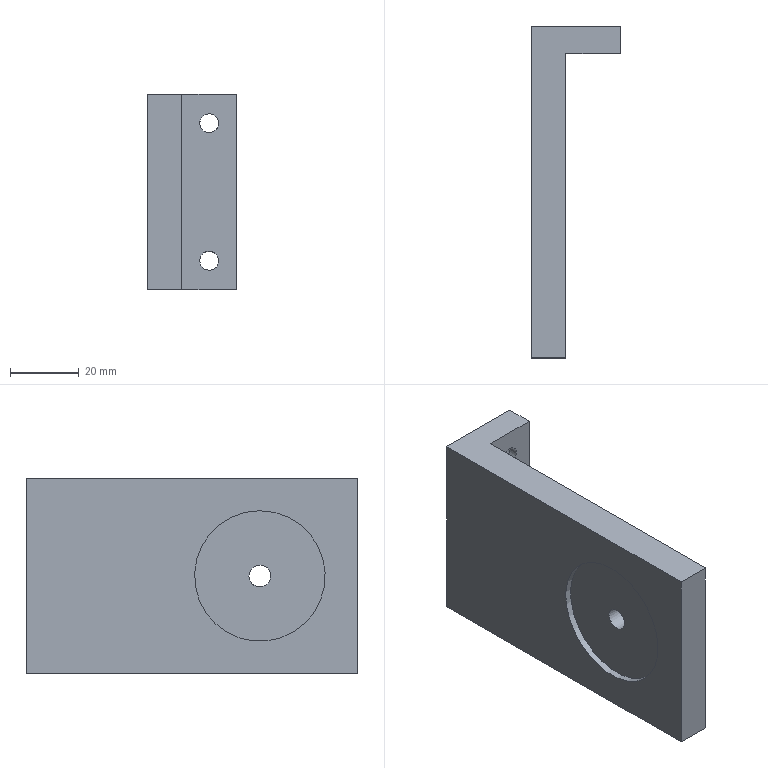Part | STEP file | 57dianjijia | 1 solid | 17 faces | box 26 x 96.5 x 57 mm | volume 58808 mm3 | plane 11 | cylinder 6 | commonest cylinder face diameters 5.5 x2 10 x2 6.35 x1 38 x1
STEP:
#1=CARTESIAN_POINT('',(0.,0.,0.));
#2=DIRECTION('',(0.,0.,1.));
#3=DIRECTION('',(1.,0.,0.));
#4=AXIS2_PLACEMENT_3D('',#1,#2,#3);
#5=CARTESIAN_POINT('',(10.,-64.825,0.));
#6=VERTEX_POINT('',#5);
#7=CARTESIAN_POINT('',(10.,-68.,0.));
#8=DIRECTION('',(1.,0.,0.));
#9=DIRECTION('',(0.,1.,0.));
#10=AXIS2_PLACEMENT_3D('',#7,#8,#9);
#11=CIRCLE('',#10,3.175);
#12=CARTESIAN_POINT('',(0.,-68.,0.));
#13=DIRECTION('',(1.,0.,0.));
#14=DIRECTION('',(0.,1.,0.));
#15=AXIS2_PLACEMENT_3D('',#12,#13,#14);
#16=CYLINDRICAL_SURFACE('',#15,3.175);
#17=CARTESIAN_POINT('',(0.,10.));
#18=DIRECTION('',(1.,0.));
#19=VECTOR('',#18,1.);
#20=LINE('',#17,#19);
#21=(GEOMETRIC_REPRESENTATION_CONTEXT(2)PARAMETRIC_REPRESENTATION_CONTEXT()REPRESENTATION_CONTEXT('',''));
#22=DEFINITIONAL_REPRESENTATION('',(#20),#21);
#23=PCURVE('',#16,#22);
#24=CARTESIAN_POINT('',(10.,-8.,28.5));
#25=DIRECTION('',(-1.,0.,0.));
#26=DIRECTION('',(0.,-1.,0.));
#27=AXIS2_PLACEMENT_3D('',#24,#25,#26);
#28=PLANE('',#27);
#29=CARTESIAN_POINT('',(56.825,-28.5));
#30=CARTESIAN_POINT('',(56.825,-23.001));
#31=CARTESIAN_POINT('',(61.587,-25.75));
#32=CARTESIAN_POINT('',(66.35,-28.5));
#33=CARTESIAN_POINT('',(61.587,-31.25));
#34=CARTESIAN_POINT('',(56.825,-33.999));
#35=CARTESIAN_POINT('',(56.825,-28.5));
#36=(BOUNDED_CURVE()B_SPLINE_CURVE(2,(#29,#30,#31,#32,#33,#34,#35),.UNSPECIFIED.,.T.,.F.)B_SPLINE_CURVE_WITH_KNOTS((1,2,2,2,2,1),(-2.094,0.,2.094,4.189,6.283,8.378),.UNSPECIFIED.)CURVE()GEOMETRIC_REPRESENTATION_ITEM()RATIONAL_B_SPLINE_CURVE((1.,0.5,1.,0.5,1.,0.5,1.))REPRESENTATION_ITEM(''));
#37=(GEOMETRIC_REPRESENTATION_CONTEXT(2)PARAMETRIC_REPRESENTATION_CONTEXT()REPRESENTATION_CONTEXT('',''));
#38=DEFINITIONAL_REPRESENTATION('',(#36),#37);
#39=PCURVE('',#28,#38);
#40=SURFACE_CURVE('',#11,(#23,#39),.PCURVE_S1.);
#41=EDGE_CURVE('',#6,#6,#40,.T.);
#42=ORIENTED_EDGE('',*,*,#41,.F.);
#43=CARTESIAN_POINT('',(2.,-64.825,0.));
#44=VERTEX_POINT('',#43);
#45=CARTESIAN_POINT('',(2.,-64.825,0.));
#46=CARTESIAN_POINT('',(10.,-64.825,0.));
#47=B_SPLINE_CURVE_WITH_KNOTS('',1,(#45,#46),.UNSPECIFIED.,.F.,.F.,(2,2),(2.,10.),.PIECEWISE_BEZIER_KNOTS.);
#48=CARTESIAN_POINT('',(0.,0.));
#49=DIRECTION('',(0.,1.));
#50=VECTOR('',#49,1.);
#51=LINE('',#48,#50);
#52=(GEOMETRIC_REPRESENTATION_CONTEXT(2)PARAMETRIC_REPRESENTATION_CONTEXT()REPRESENTATION_CONTEXT('',''));
#53=DEFINITIONAL_REPRESENTATION('',(#51),#52);
#54=PCURVE('',#16,#53);
#55=CARTESIAN_POINT('',(6.283,0.));
#56=DIRECTION('',(0.,1.));
#57=VECTOR('',#56,1.);
#58=LINE('',#55,#57);
#59=(GEOMETRIC_REPRESENTATION_CONTEXT(2)PARAMETRIC_REPRESENTATION_CONTEXT()REPRESENTATION_CONTEXT('',''));
#60=DEFINITIONAL_REPRESENTATION('',(#58),#59);
#61=PCURVE('',#16,#60);
#62=SEAM_CURVE('',#47,(#54,#61),.PCURVE_S1.);
#63=EDGE_CURVE('',#44,#6,#62,.T.);
#64=ORIENTED_EDGE('',*,*,#63,.F.);
#65=CARTESIAN_POINT('',(2.,-68.,3.175));
#66=VERTEX_POINT('',#65);
#67=CARTESIAN_POINT('',(2.,-68.,0.));
#68=DIRECTION('',(1.,0.,0.));
#69=DIRECTION('',(0.,0.,1.));
#70=AXIS2_PLACEMENT_3D('',#67,#68,#69);
#71=CIRCLE('',#70,3.175);
#72=CARTESIAN_POINT('',(-4.712,2.));
#73=DIRECTION('',(1.,0.));
#74=VECTOR('',#73,1.);
#75=LINE('',#72,#74);
#76=(GEOMETRIC_REPRESENTATION_CONTEXT(2)PARAMETRIC_REPRESENTATION_CONTEXT()REPRESENTATION_CONTEXT('',''));
#77=DEFINITIONAL_REPRESENTATION('',(#75),#76);
#78=PCURVE('',#16,#77);
#79=CARTESIAN_POINT('',(2.,-68.,0.));
#80=DIRECTION('',(-1.,0.,0.));
#81=DIRECTION('',(0.,0.,1.));
#82=AXIS2_PLACEMENT_3D('',#79,#80,#81);
#83=PLANE('',#82);
#84=CARTESIAN_POINT('',(3.175,0.));
#85=CARTESIAN_POINT('',(3.175,-5.499));
#86=CARTESIAN_POINT('',(-1.587,-2.75));
#87=CARTESIAN_POINT('',(-6.35,0.));
#88=CARTESIAN_POINT('',(-1.587,2.75));
#89=CARTESIAN_POINT('',(3.175,5.499));
#90=CARTESIAN_POINT('',(3.175,0.));
#91=(BOUNDED_CURVE()B_SPLINE_CURVE(2,(#84,#85,#86,#87,#88,#89,#90),.UNSPECIFIED.,.T.,.F.)B_SPLINE_CURVE_WITH_KNOTS((1,2,2,2,2,1),(-2.094,0.,2.094,4.189,6.283,8.378),.UNSPECIFIED.)CURVE()GEOMETRIC_REPRESENTATION_ITEM()RATIONAL_B_SPLINE_CURVE((1.,0.5,1.,0.5,1.,0.5,1.))REPRESENTATION_ITEM(''));
#92=(GEOMETRIC_REPRESENTATION_CONTEXT(2)PARAMETRIC_REPRESENTATION_CONTEXT()REPRESENTATION_CONTEXT('',''));
#93=DEFINITIONAL_REPRESENTATION('',(#91),#92);
#94=PCURVE('',#83,#93);
#95=SURFACE_CURVE('',#71,(#78,#94),.PCURVE_S1.);
#96=EDGE_CURVE('',#44,#66,#95,.T.);
#97=ORIENTED_EDGE('',*,*,#96,.T.);
#98=CARTESIAN_POINT('',(2.,-68.,0.));
#99=DIRECTION('',(1.,0.,0.));
#100=DIRECTION('',(0.,0.,1.));
#101=AXIS2_PLACEMENT_3D('',#98,#99,#100);
#102=CIRCLE('',#101,3.175);
#103=CARTESIAN_POINT('',(1.571,2.));
#104=DIRECTION('',(1.,0.));
#105=VECTOR('',#104,1.);
#106=LINE('',#103,#105);
#107=(GEOMETRIC_REPRESENTATION_CONTEXT(2)PARAMETRIC_REPRESENTATION_CONTEXT()REPRESENTATION_CONTEXT('',''));
#108=DEFINITIONAL_REPRESENTATION('',(#106),#107);
#109=PCURVE('',#16,#108);
#110=CARTESIAN_POINT('',(3.175,0.));
#111=CARTESIAN_POINT('',(3.175,-5.499));
#112=CARTESIAN_POINT('',(-1.587,-2.75));
#113=CARTESIAN_POINT('',(-6.35,0.));
#114=CARTESIAN_POINT('',(-1.587,2.75));
#115=CARTESIAN_POINT('',(3.175,5.499));
#116=CARTESIAN_POINT('',(3.175,0.));
#117=(BOUNDED_CURVE()B_SPLINE_CURVE(2,(#110,#111,#112,#113,#114,#115,#116),.UNSPECIFIED.,.T.,.F.)B_SPLINE_CURVE_WITH_KNOTS((1,2,2,2,2,1),(-2.094,0.,2.094,4.189,6.283,8.378),.UNSPECIFIED.)CURVE()GEOMETRIC_REPRESENTATION_ITEM()RATIONAL_B_SPLINE_CURVE((1.,0.5,1.,0.5,1.,0.5,1.))REPRESENTATION_ITEM(''));
#118=(GEOMETRIC_REPRESENTATION_CONTEXT(2)PARAMETRIC_REPRESENTATION_CONTEXT()REPRESENTATION_CONTEXT('',''));
#119=DEFINITIONAL_REPRESENTATION('',(#117),#118);
#120=PCURVE('',#83,#119);
#121=SURFACE_CURVE('',#102,(#109,#120),.PCURVE_S1.);
#122=EDGE_CURVE('',#66,#44,#121,.T.);
#123=ORIENTED_EDGE('',*,*,#122,.T.);
#124=ORIENTED_EDGE('',*,*,#63,.T.);
#125=EDGE_LOOP('',(#42,#64,#97,#123,#124));
#126=FACE_BOUND('',#125,.F.);
#127=ADVANCED_FACE('',(#126),#16,.F.);
#128=CARTESIAN_POINT('',(0.,-68.,19.));
#129=VERTEX_POINT('',#128);
#130=CARTESIAN_POINT('',(0.,-68.,0.));
#131=DIRECTION('',(-1.,0.,0.));
#132=DIRECTION('',(0.,0.,1.));
#133=AXIS2_PLACEMENT_3D('',#130,#131,#132);
#134=CIRCLE('',#133,19.);
#135=CARTESIAN_POINT('',(0.,-96.5,28.5));
#136=DIRECTION('',(1.,0.,0.));
#137=DIRECTION('',(0.,0.,-1.));
#138=AXIS2_PLACEMENT_3D('',#135,#136,#137);
#139=PLANE('',#138);
#140=CARTESIAN_POINT('',(9.5,28.5));
#141=CARTESIAN_POINT('',(9.5,61.409));
#142=CARTESIAN_POINT('',(38.,44.954));
#143=CARTESIAN_POINT('',(66.5,28.5));
#144=CARTESIAN_POINT('',(38.,12.046));
#145=CARTESIAN_POINT('',(9.5,-4.409));
#146=CARTESIAN_POINT('',(9.5,28.5));
#147=(BOUNDED_CURVE()B_SPLINE_CURVE(2,(#140,#141,#142,#143,#144,#145,#146),.UNSPECIFIED.,.T.,.F.)B_SPLINE_CURVE_WITH_KNOTS((1,2,2,2,2,1),(-2.094,0.,2.094,4.189,6.283,8.378),.UNSPECIFIED.)CURVE()GEOMETRIC_REPRESENTATION_ITEM()RATIONAL_B_SPLINE_CURVE((1.,0.5,1.,0.5,1.,0.5,1.))REPRESENTATION_ITEM(''));
#148=(GEOMETRIC_REPRESENTATION_CONTEXT(2)PARAMETRIC_REPRESENTATION_CONTEXT()REPRESENTATION_CONTEXT('',''));
#149=DEFINITIONAL_REPRESENTATION('',(#147),#148);
#150=PCURVE('',#139,#149);
#151=CARTESIAN_POINT('',(2.,-68.,0.));
#152=DIRECTION('',(-1.,0.,0.));
#153=DIRECTION('',(0.,0.,1.));
#154=AXIS2_PLACEMENT_3D('',#151,#152,#153);
#155=CYLINDRICAL_SURFACE('',#154,19.);
#156=CARTESIAN_POINT('',(0.,2.));
#157=DIRECTION('',(1.,0.));
#158=VECTOR('',#157,1.);
#159=LINE('',#156,#158);
#160=(GEOMETRIC_REPRESENTATION_CONTEXT(2)PARAMETRIC_REPRESENTATION_CONTEXT()REPRESENTATION_CONTEXT('',''));
#161=DEFINITIONAL_REPRESENTATION('',(#159),#160);
#162=PCURVE('',#155,#161);
#163=SURFACE_CURVE('',#134,(#150,#162),.PCURVE_S1.);
#164=EDGE_CURVE('',#129,#129,#163,.T.);
#165=ORIENTED_EDGE('',*,*,#164,.F.);
#166=EDGE_LOOP('',(#165));
#167=FACE_BOUND('',#166,.T.);
#168=CARTESIAN_POINT('',(0.,0.,-28.5));
#169=VERTEX_POINT('',#168);
#170=CARTESIAN_POINT('',(0.,-96.5,-28.5));
#171=VERTEX_POINT('',#170);
#172=CARTESIAN_POINT('',(0.,-96.5,-28.5));
#173=DIRECTION('',(0.,-1.,0.));
#174=VECTOR('',#173,1.);
#175=LINE('',#172,#174);
#176=CARTESIAN_POINT('',(57.,0.));
#177=DIRECTION('',(0.,-1.));
#178=VECTOR('',#177,1.);
#179=LINE('',#176,#178);
#180=(GEOMETRIC_REPRESENTATION_CONTEXT(2)PARAMETRIC_REPRESENTATION_CONTEXT()REPRESENTATION_CONTEXT('',''));
#181=DEFINITIONAL_REPRESENTATION('',(#179),#180);
#182=PCURVE('',#139,#181);
#183=CARTESIAN_POINT('',(0.,0.,-28.5));
#184=DIRECTION('',(0.,0.,-1.));
#185=DIRECTION('',(-1.,0.,0.));
#186=AXIS2_PLACEMENT_3D('',#183,#184,#185);
#187=PLANE('',#186);
#188=CARTESIAN_POINT('',(0.,-96.5));
#189=DIRECTION('',(0.,-1.));
#190=VECTOR('',#189,1.);
#191=LINE('',#188,#190);
#192=(GEOMETRIC_REPRESENTATION_CONTEXT(2)PARAMETRIC_REPRESENTATION_CONTEXT()REPRESENTATION_CONTEXT('',''));
#193=DEFINITIONAL_REPRESENTATION('',(#191),#192);
#194=PCURVE('',#187,#193);
#195=SURFACE_CURVE('',#175,(#182,#194),.PCURVE_S1.);
#196=EDGE_CURVE('',#169,#171,#195,.T.);
#197=ORIENTED_EDGE('',*,*,#196,.T.);
#198=CARTESIAN_POINT('',(0.,-96.5,28.5));
#199=VERTEX_POINT('',#198);
#200=CARTESIAN_POINT('',(0.,-96.5,28.5));
#201=DIRECTION('',(0.,0.,-1.));
#202=VECTOR('',#201,1.);
#203=LINE('',#200,#202);
#204=CARTESIAN_POINT('',(0.,0.));
#205=DIRECTION('',(1.,0.));
#206=VECTOR('',#205,1.);
#207=LINE('',#204,#206);
#208=(GEOMETRIC_REPRESENTATION_CONTEXT(2)PARAMETRIC_REPRESENTATION_CONTEXT()REPRESENTATION_CONTEXT('',''));
#209=DEFINITIONAL_REPRESENTATION('',(#207),#208);
#210=PCURVE('',#139,#209);
#211=CARTESIAN_POINT('',(10.,-96.5,28.5));
#212=DIRECTION('',(0.,1.,0.));
#213=DIRECTION('',(0.,0.,1.));
#214=AXIS2_PLACEMENT_3D('',#211,#212,#213);
#215=PLANE('',#214);
#216=CARTESIAN_POINT('',(0.,-10.));
#217=DIRECTION('',(-1.,0.));
#218=VECTOR('',#217,1.);
#219=LINE('',#216,#218);
#220=(GEOMETRIC_REPRESENTATION_CONTEXT(2)PARAMETRIC_REPRESENTATION_CONTEXT()REPRESENTATION_CONTEXT('',''));
#221=DEFINITIONAL_REPRESENTATION('',(#219),#220);
#222=PCURVE('',#215,#221);
#223=SURFACE_CURVE('',#203,(#210,#222),.PCURVE_S1.);
#224=EDGE_CURVE('',#199,#171,#223,.T.);
#225=ORIENTED_EDGE('',*,*,#224,.F.);
#226=CARTESIAN_POINT('',(0.,0.,28.5));
#227=VERTEX_POINT('',#226);
#228=CARTESIAN_POINT('',(0.,-96.5,28.5));
#229=DIRECTION('',(0.,-1.,0.));
#230=VECTOR('',#229,1.);
#231=LINE('',#228,#230);
#232=CARTESIAN_POINT('',(0.,0.));
#233=DIRECTION('',(0.,-1.));
#234=VECTOR('',#233,1.);
#235=LINE('',#232,#234);
#236=(GEOMETRIC_REPRESENTATION_CONTEXT(2)PARAMETRIC_REPRESENTATION_CONTEXT()REPRESENTATION_CONTEXT('',''));
#237=DEFINITIONAL_REPRESENTATION('',(#235),#236);
#238=PCURVE('',#139,#237);
#239=CARTESIAN_POINT('',(0.,0.,28.5));
#240=DIRECTION('',(0.,0.,-1.));
#241=DIRECTION('',(-1.,0.,0.));
#242=AXIS2_PLACEMENT_3D('',#239,#240,#241);
#243=PLANE('',#242);
#244=CARTESIAN_POINT('',(0.,-96.5));
#245=DIRECTION('',(0.,-1.));
#246=VECTOR('',#245,1.);
#247=LINE('',#244,#246);
#248=(GEOMETRIC_REPRESENTATION_CONTEXT(2)PARAMETRIC_REPRESENTATION_CONTEXT()REPRESENTATION_CONTEXT('',''));
#249=DEFINITIONAL_REPRESENTATION('',(#247),#248);
#250=PCURVE('',#243,#249);
#251=SURFACE_CURVE('',#231,(#238,#250),.PCURVE_S1.);
#252=EDGE_CURVE('',#227,#199,#251,.T.);
#253=ORIENTED_EDGE('',*,*,#252,.F.);
#254=CARTESIAN_POINT('',(0.,0.,28.5));
#255=DIRECTION('',(0.,0.,-1.));
#256=VECTOR('',#255,1.);
#257=LINE('',#254,#256);
#258=CARTESIAN_POINT('',(0.,96.5));
#259=DIRECTION('',(1.,0.));
#260=VECTOR('',#259,1.);
#261=LINE('',#258,#260);
#262=(GEOMETRIC_REPRESENTATION_CONTEXT(2)PARAMETRIC_REPRESENTATION_CONTEXT()REPRESENTATION_CONTEXT('',''));
#263=DEFINITIONAL_REPRESENTATION('',(#261),#262);
#264=PCURVE('',#139,#263);
#265=CARTESIAN_POINT('',(0.,0.,28.5));
#266=DIRECTION('',(0.,-1.,0.));
#267=DIRECTION('',(0.,0.,-1.));
#268=AXIS2_PLACEMENT_3D('',#265,#266,#267);
#269=PLANE('',#268);
#270=CARTESIAN_POINT('',(0.,0.));
#271=DIRECTION('',(1.,0.));
#272=VECTOR('',#271,1.);
#273=LINE('',#270,#272);
#274=(GEOMETRIC_REPRESENTATION_CONTEXT(2)PARAMETRIC_REPRESENTATION_CONTEXT()REPRESENTATION_CONTEXT('',''));
#275=DEFINITIONAL_REPRESENTATION('',(#273),#274);
#276=PCURVE('',#269,#275);
#277=SURFACE_CURVE('',#257,(#264,#276),.PCURVE_S1.);
#278=EDGE_CURVE('',#227,#169,#277,.T.);
#279=ORIENTED_EDGE('',*,*,#278,.T.);
#280=EDGE_LOOP('',(#197,#225,#253,#279));
#281=FACE_BOUND('',#280,.T.);
#282=ADVANCED_FACE('',(#167,#281),#139,.F.);
#283=CARTESIAN_POINT('',(10.,-96.5,-28.5));
#284=VERTEX_POINT('',#283);
#285=CARTESIAN_POINT('',(10.,-96.5,-28.5));
#286=DIRECTION('',(1.,0.,0.));
#287=VECTOR('',#286,1.);
#288=LINE('',#285,#287);
#289=CARTESIAN_POINT('',(-57.,0.));
#290=DIRECTION('',(0.,1.));
#291=VECTOR('',#290,1.);
#292=LINE('',#289,#291);
#293=(GEOMETRIC_REPRESENTATION_CONTEXT(2)PARAMETRIC_REPRESENTATION_CONTEXT()REPRESENTATION_CONTEXT('',''));
#294=DEFINITIONAL_REPRESENTATION('',(#292),#293);
#295=PCURVE('',#215,#294);
#296=CARTESIAN_POINT('',(-10.,-96.5));
#297=DIRECTION('',(-1.,0.));
#298=VECTOR('',#297,1.);
#299=LINE('',#296,#298);
#300=(GEOMETRIC_REPRESENTATION_CONTEXT(2)PARAMETRIC_REPRESENTATION_CONTEXT()REPRESENTATION_CONTEXT('',''));
#301=DEFINITIONAL_REPRESENTATION('',(#299),#300);
#302=PCURVE('',#187,#301);
#303=SURFACE_CURVE('',#288,(#295,#302),.PCURVE_S1.);
#304=EDGE_CURVE('',#171,#284,#303,.T.);
#305=ORIENTED_EDGE('',*,*,#304,.T.);
#306=CARTESIAN_POINT('',(10.,-96.5,28.5));
#307=VERTEX_POINT('',#306);
#308=CARTESIAN_POINT('',(10.,-96.5,28.5));
#309=DIRECTION('',(0.,0.,-1.));
#310=VECTOR('',#309,1.);
#311=LINE('',#308,#310);
#312=CARTESIAN_POINT('',(0.,0.));
#313=DIRECTION('',(-1.,0.));
#314=VECTOR('',#313,1.);
#315=LINE('',#312,#314);
#316=(GEOMETRIC_REPRESENTATION_CONTEXT(2)PARAMETRIC_REPRESENTATION_CONTEXT()REPRESENTATION_CONTEXT('',''));
#317=DEFINITIONAL_REPRESENTATION('',(#315),#316);
#318=PCURVE('',#215,#317);
#319=CARTESIAN_POINT('',(88.5,0.));
#320=DIRECTION('',(0.,-1.));
#321=VECTOR('',#320,1.);
#322=LINE('',#319,#321);
#323=(GEOMETRIC_REPRESENTATION_CONTEXT(2)PARAMETRIC_REPRESENTATION_CONTEXT()REPRESENTATION_CONTEXT('',''));
#324=DEFINITIONAL_REPRESENTATION('',(#322),#323);
#325=PCURVE('',#28,#324);
#326=SURFACE_CURVE('',#311,(#318,#325),.PCURVE_S1.);
#327=EDGE_CURVE('',#307,#284,#326,.T.);
#328=ORIENTED_EDGE('',*,*,#327,.F.);
#329=CARTESIAN_POINT('',(10.,-96.5,28.5));
#330=DIRECTION('',(1.,0.,0.));
#331=VECTOR('',#330,1.);
#332=LINE('',#329,#331);
#333=CARTESIAN_POINT('',(0.,0.));
#334=DIRECTION('',(0.,1.));
#335=VECTOR('',#334,1.);
#336=LINE('',#333,#335);
#337=(GEOMETRIC_REPRESENTATION_CONTEXT(2)PARAMETRIC_REPRESENTATION_CONTEXT()REPRESENTATION_CONTEXT('',''));
#338=DEFINITIONAL_REPRESENTATION('',(#336),#337);
#339=PCURVE('',#215,#338);
#340=CARTESIAN_POINT('',(-10.,-96.5));
#341=DIRECTION('',(-1.,0.));
#342=VECTOR('',#341,1.);
#343=LINE('',#340,#342);
#344=(GEOMETRIC_REPRESENTATION_CONTEXT(2)PARAMETRIC_REPRESENTATION_CONTEXT()REPRESENTATION_CONTEXT('',''));
#345=DEFINITIONAL_REPRESENTATION('',(#343),#344);
#346=PCURVE('',#243,#345);
#347=SURFACE_CURVE('',#332,(#339,#346),.PCURVE_S1.);
#348=EDGE_CURVE('',#199,#307,#347,.T.);
#349=ORIENTED_EDGE('',*,*,#348,.F.);
#350=ORIENTED_EDGE('',*,*,#224,.T.);
#351=EDGE_LOOP('',(#305,#328,#349,#350));
#352=FACE_BOUND('',#351,.T.);
#353=ADVANCED_FACE('',(#352),#215,.F.);
#354=ORIENTED_EDGE('',*,*,#41,.F.);
#355=EDGE_LOOP('',(#354));
#356=FACE_BOUND('',#355,.T.);
#357=CARTESIAN_POINT('',(10.,-8.,-28.5));
#358=VERTEX_POINT('',#357);
#359=CARTESIAN_POINT('',(10.,-8.,-28.5));
#360=DIRECTION('',(0.,1.,0.));
#361=VECTOR('',#360,1.);
#362=LINE('',#359,#361);
#363=CARTESIAN_POINT('',(0.,-57.));
#364=DIRECTION('',(-1.,0.));
#365=VECTOR('',#364,1.);
#366=LINE('',#363,#365);
#367=(GEOMETRIC_REPRESENTATION_CONTEXT(2)PARAMETRIC_REPRESENTATION_CONTEXT()REPRESENTATION_CONTEXT('',''));
#368=DEFINITIONAL_REPRESENTATION('',(#366),#367);
#369=PCURVE('',#28,#368);
#370=CARTESIAN_POINT('',(-10.,-8.));
#371=DIRECTION('',(0.,1.));
#372=VECTOR('',#371,1.);
#373=LINE('',#370,#372);
#374=(GEOMETRIC_REPRESENTATION_CONTEXT(2)PARAMETRIC_REPRESENTATION_CONTEXT()REPRESENTATION_CONTEXT('',''));
#375=DEFINITIONAL_REPRESENTATION('',(#373),#374);
#376=PCURVE('',#187,#375);
#377=SURFACE_CURVE('',#362,(#369,#376),.PCURVE_S1.);
#378=EDGE_CURVE('',#284,#358,#377,.T.);
#379=ORIENTED_EDGE('',*,*,#378,.T.);
#380=CARTESIAN_POINT('',(10.,-8.,28.5));
#381=VERTEX_POINT('',#380);
#382=CARTESIAN_POINT('',(10.,-8.,28.5));
#383=DIRECTION('',(0.,0.,-1.));
#384=VECTOR('',#383,1.);
#385=LINE('',#382,#384);
#386=CARTESIAN_POINT('',(0.,0.));
#387=DIRECTION('',(0.,-1.));
#388=VECTOR('',#387,1.);
#389=LINE('',#386,#388);
#390=(GEOMETRIC_REPRESENTATION_CONTEXT(2)PARAMETRIC_REPRESENTATION_CONTEXT()REPRESENTATION_CONTEXT('',''));
#391=DEFINITIONAL_REPRESENTATION('',(#389),#390);
#392=PCURVE('',#28,#391);
#393=CARTESIAN_POINT('',(26.,-8.,28.5));
#394=DIRECTION('',(0.,1.,0.));
#395=DIRECTION('',(-1.,0.,0.));
#396=AXIS2_PLACEMENT_3D('',#393,#394,#395);
#397=PLANE('',#396);
#398=CARTESIAN_POINT('',(16.,0.));
#399=DIRECTION('',(0.,-1.));
#400=VECTOR('',#399,1.);
#401=LINE('',#398,#400);
#402=(GEOMETRIC_REPRESENTATION_CONTEXT(2)PARAMETRIC_REPRESENTATION_CONTEXT()REPRESENTATION_CONTEXT('',''));
#403=DEFINITIONAL_REPRESENTATION('',(#401),#402);
#404=PCURVE('',#397,#403);
#405=SURFACE_CURVE('',#385,(#392,#404),.PCURVE_S1.);
#406=EDGE_CURVE('',#381,#358,#405,.T.);
#407=ORIENTED_EDGE('',*,*,#406,.F.);
#408=CARTESIAN_POINT('',(10.,-8.,28.5));
#409=DIRECTION('',(0.,1.,0.));
#410=VECTOR('',#409,1.);
#411=LINE('',#408,#410);
#412=CARTESIAN_POINT('',(0.,0.));
#413=DIRECTION('',(-1.,0.));
#414=VECTOR('',#413,1.);
#415=LINE('',#412,#414);
#416=(GEOMETRIC_REPRESENTATION_CONTEXT(2)PARAMETRIC_REPRESENTATION_CONTEXT()REPRESENTATION_CONTEXT('',''));
#417=DEFINITIONAL_REPRESENTATION('',(#415),#416);
#418=PCURVE('',#28,#417);
#419=CARTESIAN_POINT('',(-10.,-8.));
#420=DIRECTION('',(0.,1.));
#421=VECTOR('',#420,1.);
#422=LINE('',#419,#421);
#423=(GEOMETRIC_REPRESENTATION_CONTEXT(2)PARAMETRIC_REPRESENTATION_CONTEXT()REPRESENTATION_CONTEXT('',''));
#424=DEFINITIONAL_REPRESENTATION('',(#422),#423);
#425=PCURVE('',#243,#424);
#426=SURFACE_CURVE('',#411,(#418,#425),.PCURVE_S1.);
#427=EDGE_CURVE('',#307,#381,#426,.T.);
#428=ORIENTED_EDGE('',*,*,#427,.F.);
#429=ORIENTED_EDGE('',*,*,#327,.T.);
#430=EDGE_LOOP('',(#379,#407,#428,#429));
#431=FACE_BOUND('',#430,.T.);
#432=ADVANCED_FACE('',(#356,#431),#28,.F.);
#433=CARTESIAN_POINT('',(15.25,-8.,-20.));
#434=VERTEX_POINT('',#433);
#435=CARTESIAN_POINT('',(18.,-8.,-20.));
#436=DIRECTION('',(0.,1.,0.));
#437=DIRECTION('',(-1.,0.,0.));
#438=AXIS2_PLACEMENT_3D('',#435,#436,#437);
#439=CIRCLE('',#438,2.75);
#440=CARTESIAN_POINT('',(8.,-48.5));
#441=DIRECTION('',(1.,0.));
#442=AXIS2_PLACEMENT_2D('',#440,#441);
#443=CIRCLE('',#442,2.75);
#444=(GEOMETRIC_REPRESENTATION_CONTEXT(2)PARAMETRIC_REPRESENTATION_CONTEXT()REPRESENTATION_CONTEXT('',''));
#445=DEFINITIONAL_REPRESENTATION('',(#443),#444);
#446=PCURVE('',#397,#445);
#447=CARTESIAN_POINT('',(18.,-96.5,-20.));
#448=DIRECTION('',(0.,1.,0.));
#449=DIRECTION('',(0.,0.,1.));
#450=AXIS2_PLACEMENT_3D('',#447,#448,#449);
#451=CYLINDRICAL_SURFACE('',#450,2.75);
#452=CARTESIAN_POINT('',(4.712,88.5));
#453=DIRECTION('',(1.,0.));
#454=VECTOR('',#453,1.);
#455=LINE('',#452,#454);
#456=(GEOMETRIC_REPRESENTATION_CONTEXT(2)PARAMETRIC_REPRESENTATION_CONTEXT()REPRESENTATION_CONTEXT('',''));
#457=DEFINITIONAL_REPRESENTATION('',(#455),#456);
#458=PCURVE('',#451,#457);
#459=SURFACE_CURVE('',#439,(#446,#458),.PCURVE_S1.);
#460=EDGE_CURVE('',#434,#434,#459,.T.);
#461=ORIENTED_EDGE('',*,*,#460,.T.);
#462=EDGE_LOOP('',(#461));
#463=FACE_BOUND('',#462,.T.);
#464=CARTESIAN_POINT('',(15.25,-8.,20.));
#465=VERTEX_POINT('',#464);
#466=CARTESIAN_POINT('',(18.,-8.,22.75));
#467=VERTEX_POINT('',#466);
#468=CARTESIAN_POINT('',(18.,-8.,20.));
#469=DIRECTION('',(0.,1.,0.));
#470=DIRECTION('',(-1.,0.,0.));
#471=AXIS2_PLACEMENT_3D('',#468,#469,#470);
#472=CIRCLE('',#471,2.75);
#473=CARTESIAN_POINT('',(8.,-8.5));
#474=DIRECTION('',(1.,0.));
#475=AXIS2_PLACEMENT_2D('',#473,#474);
#476=CIRCLE('',#475,2.75);
#477=(GEOMETRIC_REPRESENTATION_CONTEXT(2)PARAMETRIC_REPRESENTATION_CONTEXT()REPRESENTATION_CONTEXT('',''));
#478=DEFINITIONAL_REPRESENTATION('',(#476),#477);
#479=PCURVE('',#397,#478);
#480=CARTESIAN_POINT('',(18.,-96.5,20.));
#481=DIRECTION('',(0.,1.,0.));
#482=DIRECTION('',(0.,0.,1.));
#483=AXIS2_PLACEMENT_3D('',#480,#481,#482);
#484=CYLINDRICAL_SURFACE('',#483,2.75);
#485=CARTESIAN_POINT('',(4.712,88.5));
#486=DIRECTION('',(1.,0.));
#487=VECTOR('',#486,1.);
#488=LINE('',#485,#487);
#489=(GEOMETRIC_REPRESENTATION_CONTEXT(2)PARAMETRIC_REPRESENTATION_CONTEXT()REPRESENTATION_CONTEXT('',''));
#490=DEFINITIONAL_REPRESENTATION('',(#488),#489);
#491=PCURVE('',#484,#490);
#492=SURFACE_CURVE('',#472,(#479,#491),.PCURVE_S1.);
#493=EDGE_CURVE('',#465,#467,#492,.T.);
#494=ORIENTED_EDGE('',*,*,#493,.T.);
#495=CARTESIAN_POINT('',(18.,-8.,20.));
#496=DIRECTION('',(0.,1.,0.));
#497=DIRECTION('',(-1.,0.,0.));
#498=AXIS2_PLACEMENT_3D('',#495,#496,#497);
#499=CIRCLE('',#498,2.75);
#500=CARTESIAN_POINT('',(8.,-8.5));
#501=DIRECTION('',(1.,0.));
#502=AXIS2_PLACEMENT_2D('',#500,#501);
#503=CIRCLE('',#502,2.75);
#504=(GEOMETRIC_REPRESENTATION_CONTEXT(2)PARAMETRIC_REPRESENTATION_CONTEXT()REPRESENTATION_CONTEXT('',''));
#505=DEFINITIONAL_REPRESENTATION('',(#503),#504);
#506=PCURVE('',#397,#505);
#507=CARTESIAN_POINT('',(-1.571,88.5));
#508=DIRECTION('',(1.,0.));
#509=VECTOR('',#508,1.);
#510=LINE('',#507,#509);
#511=(GEOMETRIC_REPRESENTATION_CONTEXT(2)PARAMETRIC_REPRESENTATION_CONTEXT()REPRESENTATION_CONTEXT('',''));
#512=DEFINITIONAL_REPRESENTATION('',(#510),#511);
#513=PCURVE('',#484,#512);
#514=SURFACE_CURVE('',#499,(#506,#513),.PCURVE_S1.);
#515=EDGE_CURVE('',#467,#465,#514,.T.);
#516=ORIENTED_EDGE('',*,*,#515,.T.);
#517=EDGE_LOOP('',(#494,#516));
#518=FACE_BOUND('',#517,.T.);
#519=CARTESIAN_POINT('',(26.,-8.,-28.5));
#520=VERTEX_POINT('',#519);
#521=CARTESIAN_POINT('',(26.,-8.,-28.5));
#522=DIRECTION('',(1.,0.,0.));
#523=VECTOR('',#522,1.);
#524=LINE('',#521,#523);
#525=CARTESIAN_POINT('',(0.,-57.));
#526=DIRECTION('',(-1.,0.));
#527=VECTOR('',#526,1.);
#528=LINE('',#525,#527);
#529=(GEOMETRIC_REPRESENTATION_CONTEXT(2)PARAMETRIC_REPRESENTATION_CONTEXT()REPRESENTATION_CONTEXT('',''));
#530=DEFINITIONAL_REPRESENTATION('',(#528),#529);
#531=PCURVE('',#397,#530);
#532=CARTESIAN_POINT('',(-26.,-8.));
#533=DIRECTION('',(-1.,0.));
#534=VECTOR('',#533,1.);
#535=LINE('',#532,#534);
#536=(GEOMETRIC_REPRESENTATION_CONTEXT(2)PARAMETRIC_REPRESENTATION_CONTEXT()REPRESENTATION_CONTEXT('',''));
#537=DEFINITIONAL_REPRESENTATION('',(#535),#536);
#538=PCURVE('',#187,#537);
#539=SURFACE_CURVE('',#524,(#531,#538),.PCURVE_S1.);
#540=EDGE_CURVE('',#358,#520,#539,.T.);
#541=ORIENTED_EDGE('',*,*,#540,.T.);
#542=CARTESIAN_POINT('',(26.,-8.,28.5));
#543=VERTEX_POINT('',#542);
#544=CARTESIAN_POINT('',(26.,-8.,28.5));
#545=DIRECTION('',(0.,0.,-1.));
#546=VECTOR('',#545,1.);
#547=LINE('',#544,#546);
#548=CARTESIAN_POINT('',(0.,0.));
#549=DIRECTION('',(0.,-1.));
#550=VECTOR('',#549,1.);
#551=LINE('',#548,#550);
#552=(GEOMETRIC_REPRESENTATION_CONTEXT(2)PARAMETRIC_REPRESENTATION_CONTEXT()REPRESENTATION_CONTEXT('',''));
#553=DEFINITIONAL_REPRESENTATION('',(#551),#552);
#554=PCURVE('',#397,#553);
#555=CARTESIAN_POINT('',(26.,0.,28.5));
#556=DIRECTION('',(-1.,0.,0.));
#557=DIRECTION('',(0.,0.,1.));
#558=AXIS2_PLACEMENT_3D('',#555,#556,#557);
#559=PLANE('',#558);
#560=CARTESIAN_POINT('',(0.,-8.));
#561=DIRECTION('',(-1.,0.));
#562=VECTOR('',#561,1.);
#563=LINE('',#560,#562);
#564=(GEOMETRIC_REPRESENTATION_CONTEXT(2)PARAMETRIC_REPRESENTATION_CONTEXT()REPRESENTATION_CONTEXT('',''));
#565=DEFINITIONAL_REPRESENTATION('',(#563),#564);
#566=PCURVE('',#559,#565);
#567=SURFACE_CURVE('',#547,(#554,#566),.PCURVE_S1.);
#568=EDGE_CURVE('',#543,#520,#567,.T.);
#569=ORIENTED_EDGE('',*,*,#568,.F.);
#570=CARTESIAN_POINT('',(26.,-8.,28.5));
#571=DIRECTION('',(1.,0.,0.));
#572=VECTOR('',#571,1.);
#573=LINE('',#570,#572);
#574=CARTESIAN_POINT('',(0.,0.));
#575=DIRECTION('',(-1.,0.));
#576=VECTOR('',#575,1.);
#577=LINE('',#574,#576);
#578=(GEOMETRIC_REPRESENTATION_CONTEXT(2)PARAMETRIC_REPRESENTATION_CONTEXT()REPRESENTATION_CONTEXT('',''));
#579=DEFINITIONAL_REPRESENTATION('',(#577),#578);
#580=PCURVE('',#397,#579);
#581=CARTESIAN_POINT('',(-26.,-8.));
#582=DIRECTION('',(-1.,0.));
#583=VECTOR('',#582,1.);
#584=LINE('',#581,#583);
#585=(GEOMETRIC_REPRESENTATION_CONTEXT(2)PARAMETRIC_REPRESENTATION_CONTEXT()REPRESENTATION_CONTEXT('',''));
#586=DEFINITIONAL_REPRESENTATION('',(#584),#585);
#587=PCURVE('',#243,#586);
#588=SURFACE_CURVE('',#573,(#580,#587),.PCURVE_S1.);
#589=EDGE_CURVE('',#381,#543,#588,.T.);
#590=ORIENTED_EDGE('',*,*,#589,.F.);
#591=ORIENTED_EDGE('',*,*,#406,.T.);
#592=EDGE_LOOP('',(#541,#569,#590,#591));
#593=FACE_BOUND('',#592,.T.);
#594=ADVANCED_FACE('',(#463,#518,#593),#397,.F.);
#595=CARTESIAN_POINT('',(26.,0.,-28.5));
#596=VERTEX_POINT('',#595);
#597=CARTESIAN_POINT('',(26.,0.,-28.5));
#598=DIRECTION('',(0.,1.,0.));
#599=VECTOR('',#598,1.);
#600=LINE('',#597,#599);
#601=CARTESIAN_POINT('',(-57.,0.));
#602=DIRECTION('',(0.,1.));
#603=VECTOR('',#602,1.);
#604=LINE('',#601,#603);
#605=(GEOMETRIC_REPRESENTATION_CONTEXT(2)PARAMETRIC_REPRESENTATION_CONTEXT()REPRESENTATION_CONTEXT('',''));
#606=DEFINITIONAL_REPRESENTATION('',(#604),#605);
#607=PCURVE('',#559,#606);
#608=CARTESIAN_POINT('',(-26.,0.));
#609=DIRECTION('',(0.,1.));
#610=VECTOR('',#609,1.);
#611=LINE('',#608,#610);
#612=(GEOMETRIC_REPRESENTATION_CONTEXT(2)PARAMETRIC_REPRESENTATION_CONTEXT()REPRESENTATION_CONTEXT('',''));
#613=DEFINITIONAL_REPRESENTATION('',(#611),#612);
#614=PCURVE('',#187,#613);
#615=SURFACE_CURVE('',#600,(#607,#614),.PCURVE_S1.);
#616=EDGE_CURVE('',#520,#596,#615,.T.);
#617=ORIENTED_EDGE('',*,*,#616,.T.);
#618=CARTESIAN_POINT('',(26.,0.,28.5));
#619=VERTEX_POINT('',#618);
#620=CARTESIAN_POINT('',(26.,0.,28.5));
#621=DIRECTION('',(0.,0.,-1.));
#622=VECTOR('',#621,1.);
#623=LINE('',#620,#622);
#624=CARTESIAN_POINT('',(0.,0.));
#625=DIRECTION('',(-1.,0.));
#626=VECTOR('',#625,1.);
#627=LINE('',#624,#626);
#628=(GEOMETRIC_REPRESENTATION_CONTEXT(2)PARAMETRIC_REPRESENTATION_CONTEXT()REPRESENTATION_CONTEXT('',''));
#629=DEFINITIONAL_REPRESENTATION('',(#627),#628);
#630=PCURVE('',#559,#629);
#631=CARTESIAN_POINT('',(0.,26.));
#632=DIRECTION('',(1.,0.));
#633=VECTOR('',#632,1.);
#634=LINE('',#631,#633);
#635=(GEOMETRIC_REPRESENTATION_CONTEXT(2)PARAMETRIC_REPRESENTATION_CONTEXT()REPRESENTATION_CONTEXT('',''));
#636=DEFINITIONAL_REPRESENTATION('',(#634),#635);
#637=PCURVE('',#269,#636);
#638=SURFACE_CURVE('',#623,(#630,#637),.PCURVE_S1.);
#639=EDGE_CURVE('',#619,#596,#638,.T.);
#640=ORIENTED_EDGE('',*,*,#639,.F.);
#641=CARTESIAN_POINT('',(26.,0.,28.5));
#642=DIRECTION('',(0.,1.,0.));
#643=VECTOR('',#642,1.);
#644=LINE('',#641,#643);
#645=CARTESIAN_POINT('',(0.,0.));
#646=DIRECTION('',(0.,1.));
#647=VECTOR('',#646,1.);
#648=LINE('',#645,#647);
#649=(GEOMETRIC_REPRESENTATION_CONTEXT(2)PARAMETRIC_REPRESENTATION_CONTEXT()REPRESENTATION_CONTEXT('',''));
#650=DEFINITIONAL_REPRESENTATION('',(#648),#649);
#651=PCURVE('',#559,#650);
#652=CARTESIAN_POINT('',(-26.,0.));
#653=DIRECTION('',(0.,1.));
#654=VECTOR('',#653,1.);
#655=LINE('',#652,#654);
#656=(GEOMETRIC_REPRESENTATION_CONTEXT(2)PARAMETRIC_REPRESENTATION_CONTEXT()REPRESENTATION_CONTEXT('',''));
#657=DEFINITIONAL_REPRESENTATION('',(#655),#656);
#658=PCURVE('',#243,#657);
#659=SURFACE_CURVE('',#644,(#651,#658),.PCURVE_S1.);
#660=EDGE_CURVE('',#543,#619,#659,.T.);
#661=ORIENTED_EDGE('',*,*,#660,.F.);
#662=ORIENTED_EDGE('',*,*,#568,.T.);
#663=EDGE_LOOP('',(#617,#640,#661,#662));
#664=FACE_BOUND('',#663,.T.);
#665=ADVANCED_FACE('',(#664),#559,.F.);
#666=CARTESIAN_POINT('',(18.,0.,-25.));
#667=VERTEX_POINT('',#666);
#668=CARTESIAN_POINT('',(18.,0.,-20.));
#669=DIRECTION('',(0.,1.,0.));
#670=DIRECTION('',(0.,0.,-1.));
#671=AXIS2_PLACEMENT_3D('',#668,#669,#670);
#672=CIRCLE('',#671,5.);
#673=CARTESIAN_POINT('',(53.5,18.));
#674=CARTESIAN_POINT('',(53.5,9.34));
#675=CARTESIAN_POINT('',(46.,13.67));
#676=CARTESIAN_POINT('',(38.5,18.));
#677=CARTESIAN_POINT('',(46.,22.33));
#678=CARTESIAN_POINT('',(53.5,26.66));
#679=CARTESIAN_POINT('',(53.5,18.));
#680=(BOUNDED_CURVE()B_SPLINE_CURVE(2,(#673,#674,#675,#676,#677,#678,#679),.UNSPECIFIED.,.T.,.F.)B_SPLINE_CURVE_WITH_KNOTS((1,2,2,2,2,1),(-2.094,0.,2.094,4.189,6.283,8.378),.UNSPECIFIED.)CURVE()GEOMETRIC_REPRESENTATION_ITEM()RATIONAL_B_SPLINE_CURVE((1.,0.5,1.,0.5,1.,0.5,1.))REPRESENTATION_ITEM(''));
#681=(GEOMETRIC_REPRESENTATION_CONTEXT(2)PARAMETRIC_REPRESENTATION_CONTEXT()REPRESENTATION_CONTEXT('',''));
#682=DEFINITIONAL_REPRESENTATION('',(#680),#681);
#683=PCURVE('',#269,#682);
#684=CARTESIAN_POINT('',(18.,-5.4,-20.));
#685=DIRECTION('',(0.,1.,0.));
#686=DIRECTION('',(0.,0.,1.));
#687=AXIS2_PLACEMENT_3D('',#684,#685,#686);
#688=CYLINDRICAL_SURFACE('',#687,5.);
#689=CARTESIAN_POINT('',(3.142,5.4));
#690=DIRECTION('',(1.,0.));
#691=VECTOR('',#690,1.);
#692=LINE('',#689,#691);
#693=(GEOMETRIC_REPRESENTATION_CONTEXT(2)PARAMETRIC_REPRESENTATION_CONTEXT()REPRESENTATION_CONTEXT('',''));
#694=DEFINITIONAL_REPRESENTATION('',(#692),#693);
#695=PCURVE('',#688,#694);
#696=SURFACE_CURVE('',#672,(#683,#695),.PCURVE_S1.);
#697=EDGE_CURVE('',#667,#667,#696,.T.);
#698=ORIENTED_EDGE('',*,*,#697,.F.);
#699=EDGE_LOOP('',(#698));
#700=FACE_BOUND('',#699,.T.);
#701=CARTESIAN_POINT('',(18.,0.,25.));
#702=VERTEX_POINT('',#701);
#703=CARTESIAN_POINT('',(18.,0.,20.));
#704=DIRECTION('',(0.,1.,0.));
#705=DIRECTION('',(0.,0.,1.));
#706=AXIS2_PLACEMENT_3D('',#703,#704,#705);
#707=CIRCLE('',#706,5.);
#708=CARTESIAN_POINT('',(3.5,18.));
#709=CARTESIAN_POINT('',(3.5,26.66));
#710=CARTESIAN_POINT('',(11.,22.33));
#711=CARTESIAN_POINT('',(18.5,18.));
#712=CARTESIAN_POINT('',(11.,13.67));
#713=CARTESIAN_POINT('',(3.5,9.34));
#714=CARTESIAN_POINT('',(3.5,18.));
#715=(BOUNDED_CURVE()B_SPLINE_CURVE(2,(#708,#709,#710,#711,#712,#713,#714),.UNSPECIFIED.,.T.,.F.)B_SPLINE_CURVE_WITH_KNOTS((1,2,2,2,2,1),(-2.094,0.,2.094,4.189,6.283,8.378),.UNSPECIFIED.)CURVE()GEOMETRIC_REPRESENTATION_ITEM()RATIONAL_B_SPLINE_CURVE((1.,0.5,1.,0.5,1.,0.5,1.))REPRESENTATION_ITEM(''));
#716=(GEOMETRIC_REPRESENTATION_CONTEXT(2)PARAMETRIC_REPRESENTATION_CONTEXT()REPRESENTATION_CONTEXT('',''));
#717=DEFINITIONAL_REPRESENTATION('',(#715),#716);
#718=PCURVE('',#269,#717);
#719=CARTESIAN_POINT('',(18.,-5.4,20.));
#720=DIRECTION('',(0.,1.,0.));
#721=DIRECTION('',(0.,0.,1.));
#722=AXIS2_PLACEMENT_3D('',#719,#720,#721);
#723=CYLINDRICAL_SURFACE('',#722,5.);
#724=CARTESIAN_POINT('',(0.,5.4));
#725=DIRECTION('',(1.,0.));
#726=VECTOR('',#725,1.);
#727=LINE('',#724,#726);
#728=(GEOMETRIC_REPRESENTATION_CONTEXT(2)PARAMETRIC_REPRESENTATION_CONTEXT()REPRESENTATION_CONTEXT('',''));
#729=DEFINITIONAL_REPRESENTATION('',(#727),#728);
#730=PCURVE('',#723,#729);
#731=SURFACE_CURVE('',#707,(#718,#730),.PCURVE_S1.);
#732=EDGE_CURVE('',#702,#702,#731,.T.);
#733=ORIENTED_EDGE('',*,*,#732,.F.);
#734=EDGE_LOOP('',(#733));
#735=FACE_BOUND('',#734,.T.);
#736=CARTESIAN_POINT('',(0.,0.,-28.5));
#737=DIRECTION('',(-1.,0.,0.));
#738=VECTOR('',#737,1.);
#739=LINE('',#736,#738);
#740=CARTESIAN_POINT('',(57.,0.));
#741=DIRECTION('',(0.,-1.));
#742=VECTOR('',#741,1.);
#743=LINE('',#740,#742);
#744=(GEOMETRIC_REPRESENTATION_CONTEXT(2)PARAMETRIC_REPRESENTATION_CONTEXT()REPRESENTATION_CONTEXT('',''));
#745=DEFINITIONAL_REPRESENTATION('',(#743),#744);
#746=PCURVE('',#269,#745);
#747=CARTESIAN_POINT('',(0.,0.));
#748=DIRECTION('',(1.,0.));
#749=VECTOR('',#748,1.);
#750=LINE('',#747,#749);
#751=(GEOMETRIC_REPRESENTATION_CONTEXT(2)PARAMETRIC_REPRESENTATION_CONTEXT()REPRESENTATION_CONTEXT('',''));
#752=DEFINITIONAL_REPRESENTATION('',(#750),#751);
#753=PCURVE('',#187,#752);
#754=SURFACE_CURVE('',#739,(#746,#753),.PCURVE_S1.);
#755=EDGE_CURVE('',#596,#169,#754,.T.);
#756=ORIENTED_EDGE('',*,*,#755,.T.);
#757=ORIENTED_EDGE('',*,*,#278,.F.);
#758=CARTESIAN_POINT('',(0.,0.,28.5));
#759=DIRECTION('',(-1.,0.,0.));
#760=VECTOR('',#759,1.);
#761=LINE('',#758,#760);
#762=CARTESIAN_POINT('',(0.,0.));
#763=DIRECTION('',(0.,-1.));
#764=VECTOR('',#763,1.);
#765=LINE('',#762,#764);
#766=(GEOMETRIC_REPRESENTATION_CONTEXT(2)PARAMETRIC_REPRESENTATION_CONTEXT()REPRESENTATION_CONTEXT('',''));
#767=DEFINITIONAL_REPRESENTATION('',(#765),#766);
#768=PCURVE('',#269,#767);
#769=CARTESIAN_POINT('',(0.,0.));
#770=DIRECTION('',(1.,0.));
#771=VECTOR('',#770,1.);
#772=LINE('',#769,#771);
#773=(GEOMETRIC_REPRESENTATION_CONTEXT(2)PARAMETRIC_REPRESENTATION_CONTEXT()REPRESENTATION_CONTEXT('',''));
#774=DEFINITIONAL_REPRESENTATION('',(#772),#773);
#775=PCURVE('',#243,#774);
#776=SURFACE_CURVE('',#761,(#768,#775),.PCURVE_S1.);
#777=EDGE_CURVE('',#619,#227,#776,.T.);
#778=ORIENTED_EDGE('',*,*,#777,.F.);
#779=ORIENTED_EDGE('',*,*,#639,.T.);
#780=EDGE_LOOP('',(#756,#757,#778,#779));
#781=FACE_BOUND('',#780,.T.);
#782=ADVANCED_FACE('',(#700,#735,#781),#269,.F.);
#783=ORIENTED_EDGE('',*,*,#252,.T.);
#784=ORIENTED_EDGE('',*,*,#348,.T.);
#785=ORIENTED_EDGE('',*,*,#427,.T.);
#786=ORIENTED_EDGE('',*,*,#589,.T.);
#787=ORIENTED_EDGE('',*,*,#660,.T.);
#788=ORIENTED_EDGE('',*,*,#777,.T.);
#789=EDGE_LOOP('',(#783,#784,#785,#786,#787,#788));
#790=FACE_BOUND('',#789,.T.);
#791=ADVANCED_FACE('',(#790),#243,.F.);
#792=ORIENTED_EDGE('',*,*,#196,.F.);
#793=ORIENTED_EDGE('',*,*,#755,.F.);
#794=ORIENTED_EDGE('',*,*,#616,.F.);
#795=ORIENTED_EDGE('',*,*,#540,.F.);
#796=ORIENTED_EDGE('',*,*,#378,.F.);
#797=ORIENTED_EDGE('',*,*,#304,.F.);
#798=EDGE_LOOP('',(#792,#793,#794,#795,#796,#797));
#799=FACE_BOUND('',#798,.T.);
#800=ADVANCED_FACE('',(#799),#187,.T.);
#801=CARTESIAN_POINT('',(18.,-5.4,25.));
#802=VERTEX_POINT('',#801);
#803=CARTESIAN_POINT('',(18.,-5.4,20.));
#804=DIRECTION('',(0.,1.,0.));
#805=DIRECTION('',(0.,0.,1.));
#806=AXIS2_PLACEMENT_3D('',#803,#804,#805);
#807=CIRCLE('',#806,5.);
#808=CARTESIAN_POINT('',(0.,0.));
#809=DIRECTION('',(1.,0.));
#810=VECTOR('',#809,1.);
#811=LINE('',#808,#810);
#812=(GEOMETRIC_REPRESENTATION_CONTEXT(2)PARAMETRIC_REPRESENTATION_CONTEXT()REPRESENTATION_CONTEXT('',''));
#813=DEFINITIONAL_REPRESENTATION('',(#811),#812);
#814=PCURVE('',#723,#813);
#815=CARTESIAN_POINT('',(18.,-5.4,20.));
#816=DIRECTION('',(0.,1.,0.));
#817=DIRECTION('',(0.,0.,1.));
#818=AXIS2_PLACEMENT_3D('',#815,#816,#817);
#819=PLANE('',#818);
#820=CARTESIAN_POINT('',(0.,0.));
#821=DIRECTION('',(1.,0.));
#822=AXIS2_PLACEMENT_2D('',#820,#821);
#823=CIRCLE('',#822,5.);
#824=(GEOMETRIC_REPRESENTATION_CONTEXT(2)PARAMETRIC_REPRESENTATION_CONTEXT()REPRESENTATION_CONTEXT('',''));
#825=DEFINITIONAL_REPRESENTATION('',(#823),#824);
#826=PCURVE('',#819,#825);
#827=SURFACE_CURVE('',#807,(#814,#826),.PCURVE_S1.);
#828=EDGE_CURVE('',#802,#802,#827,.T.);
#829=ORIENTED_EDGE('',*,*,#828,.T.);
#830=CARTESIAN_POINT('',(18.,-5.4,25.));
#831=CARTESIAN_POINT('',(18.,0.,25.));
#832=B_SPLINE_CURVE_WITH_KNOTS('',1,(#830,#831),.UNSPECIFIED.,.F.,.F.,(2,2),(0.,5.4),.PIECEWISE_BEZIER_KNOTS.);
#833=CARTESIAN_POINT('',(6.283,0.));
#834=DIRECTION('',(0.,1.));
#835=VECTOR('',#834,1.);
#836=LINE('',#833,#835);
#837=(GEOMETRIC_REPRESENTATION_CONTEXT(2)PARAMETRIC_REPRESENTATION_CONTEXT()REPRESENTATION_CONTEXT('',''));
#838=DEFINITIONAL_REPRESENTATION('',(#836),#837);
#839=PCURVE('',#723,#838);
#840=CARTESIAN_POINT('',(0.,0.));
#841=DIRECTION('',(0.,1.));
#842=VECTOR('',#841,1.);
#843=LINE('',#840,#842);
#844=(GEOMETRIC_REPRESENTATION_CONTEXT(2)PARAMETRIC_REPRESENTATION_CONTEXT()REPRESENTATION_CONTEXT('',''));
#845=DEFINITIONAL_REPRESENTATION('',(#843),#844);
#846=PCURVE('',#723,#845);
#847=SEAM_CURVE('',#832,(#839,#846),.PCURVE_S1.);
#848=EDGE_CURVE('',#802,#702,#847,.T.);
#849=ORIENTED_EDGE('',*,*,#848,.T.);
#850=ORIENTED_EDGE('',*,*,#732,.F.);
#851=ORIENTED_EDGE('',*,*,#848,.F.);
#852=EDGE_LOOP('',(#829,#849,#850,#851));
#853=FACE_BOUND('',#852,.F.);
#854=ADVANCED_FACE('',(#853),#723,.F.);
#855=CARTESIAN_POINT('',(18.,-5.4,22.75));
#856=VERTEX_POINT('',#855);
#857=CARTESIAN_POINT('',(18.,-5.4,20.));
#858=DIRECTION('',(0.,1.,0.));
#859=DIRECTION('',(0.,0.,1.));
#860=AXIS2_PLACEMENT_3D('',#857,#858,#859);
#861=CIRCLE('',#860,2.75);
#862=CARTESIAN_POINT('',(0.,0.));
#863=DIRECTION('',(1.,0.));
#864=AXIS2_PLACEMENT_2D('',#862,#863);
#865=CIRCLE('',#864,2.75);
#866=(GEOMETRIC_REPRESENTATION_CONTEXT(2)PARAMETRIC_REPRESENTATION_CONTEXT()REPRESENTATION_CONTEXT('',''));
#867=DEFINITIONAL_REPRESENTATION('',(#865),#866);
#868=PCURVE('',#819,#867);
#869=CARTESIAN_POINT('',(0.,91.1));
#870=DIRECTION('',(1.,0.));
#871=VECTOR('',#870,1.);
#872=LINE('',#869,#871);
#873=(GEOMETRIC_REPRESENTATION_CONTEXT(2)PARAMETRIC_REPRESENTATION_CONTEXT()REPRESENTATION_CONTEXT('',''));
#874=DEFINITIONAL_REPRESENTATION('',(#872),#873);
#875=PCURVE('',#484,#874);
#876=SURFACE_CURVE('',#861,(#868,#875),.PCURVE_S1.);
#877=EDGE_CURVE('',#856,#856,#876,.T.);
#878=ORIENTED_EDGE('',*,*,#877,.F.);
#879=EDGE_LOOP('',(#878));
#880=FACE_BOUND('',#879,.T.);
#881=ORIENTED_EDGE('',*,*,#828,.T.);
#882=EDGE_LOOP('',(#881));
#883=FACE_BOUND('',#882,.T.);
#884=ADVANCED_FACE('',(#880,#883),#819,.T.);
#885=CARTESIAN_POINT('',(18.,-5.4,-25.));
#886=VERTEX_POINT('',#885);
#887=CARTESIAN_POINT('',(18.,-5.4,-20.));
#888=DIRECTION('',(0.,1.,0.));
#889=DIRECTION('',(0.,0.,-1.));
#890=AXIS2_PLACEMENT_3D('',#887,#888,#889);
#891=CIRCLE('',#890,5.);
#892=CARTESIAN_POINT('',(3.142,0.));
#893=DIRECTION('',(1.,0.));
#894=VECTOR('',#893,1.);
#895=LINE('',#892,#894);
#896=(GEOMETRIC_REPRESENTATION_CONTEXT(2)PARAMETRIC_REPRESENTATION_CONTEXT()REPRESENTATION_CONTEXT('',''));
#897=DEFINITIONAL_REPRESENTATION('',(#895),#896);
#898=PCURVE('',#688,#897);
#899=CARTESIAN_POINT('',(18.,-5.4,-20.));
#900=DIRECTION('',(0.,-1.,0.));
#901=DIRECTION('',(0.,0.,-1.));
#902=AXIS2_PLACEMENT_3D('',#899,#900,#901);
#903=PLANE('',#902);
#904=CARTESIAN_POINT('',(5.,0.));
#905=CARTESIAN_POINT('',(5.,-8.66));
#906=CARTESIAN_POINT('',(-2.5,-4.33));
#907=CARTESIAN_POINT('',(-10.,0.));
#908=CARTESIAN_POINT('',(-2.5,4.33));
#909=CARTESIAN_POINT('',(5.,8.66));
#910=CARTESIAN_POINT('',(5.,0.));
#911=(BOUNDED_CURVE()B_SPLINE_CURVE(2,(#904,#905,#906,#907,#908,#909,#910),.UNSPECIFIED.,.T.,.F.)B_SPLINE_CURVE_WITH_KNOTS((1,2,2,2,2,1),(-2.094,0.,2.094,4.189,6.283,8.378),.UNSPECIFIED.)CURVE()GEOMETRIC_REPRESENTATION_ITEM()RATIONAL_B_SPLINE_CURVE((1.,0.5,1.,0.5,1.,0.5,1.))REPRESENTATION_ITEM(''));
#912=(GEOMETRIC_REPRESENTATION_CONTEXT(2)PARAMETRIC_REPRESENTATION_CONTEXT()REPRESENTATION_CONTEXT('',''));
#913=DEFINITIONAL_REPRESENTATION('',(#911),#912);
#914=PCURVE('',#903,#913);
#915=SURFACE_CURVE('',#891,(#898,#914),.PCURVE_S1.);
#916=EDGE_CURVE('',#886,#886,#915,.T.);
#917=ORIENTED_EDGE('',*,*,#916,.T.);
#918=CARTESIAN_POINT('',(18.,-5.4,-25.));
#919=CARTESIAN_POINT('',(18.,0.,-25.));
#920=B_SPLINE_CURVE_WITH_KNOTS('',1,(#918,#919),.UNSPECIFIED.,.F.,.F.,(2,2),(0.,5.4),.PIECEWISE_BEZIER_KNOTS.);
#921=CARTESIAN_POINT('',(9.425,0.));
#922=DIRECTION('',(0.,1.));
#923=VECTOR('',#922,1.);
#924=LINE('',#921,#923);
#925=(GEOMETRIC_REPRESENTATION_CONTEXT(2)PARAMETRIC_REPRESENTATION_CONTEXT()REPRESENTATION_CONTEXT('',''));
#926=DEFINITIONAL_REPRESENTATION('',(#924),#925);
#927=PCURVE('',#688,#926);
#928=CARTESIAN_POINT('',(3.142,0.));
#929=DIRECTION('',(0.,1.));
#930=VECTOR('',#929,1.);
#931=LINE('',#928,#930);
#932=(GEOMETRIC_REPRESENTATION_CONTEXT(2)PARAMETRIC_REPRESENTATION_CONTEXT()REPRESENTATION_CONTEXT('',''));
#933=DEFINITIONAL_REPRESENTATION('',(#931),#932);
#934=PCURVE('',#688,#933);
#935=SEAM_CURVE('',#920,(#927,#934),.PCURVE_S1.);
#936=EDGE_CURVE('',#886,#667,#935,.T.);
#937=ORIENTED_EDGE('',*,*,#936,.T.);
#938=ORIENTED_EDGE('',*,*,#697,.F.);
#939=ORIENTED_EDGE('',*,*,#936,.F.);
#940=EDGE_LOOP('',(#917,#937,#938,#939));
#941=FACE_BOUND('',#940,.F.);
#942=ADVANCED_FACE('',(#941),#688,.F.);
#943=CARTESIAN_POINT('',(18.,-5.4,-22.75));
#944=VERTEX_POINT('',#943);
#945=CARTESIAN_POINT('',(15.25,-5.4,-20.));
#946=VERTEX_POINT('',#945);
#947=CARTESIAN_POINT('',(18.,-5.4,-20.));
#948=DIRECTION('',(0.,1.,0.));
#949=DIRECTION('',(0.,0.,-1.));
#950=AXIS2_PLACEMENT_3D('',#947,#948,#949);
#951=CIRCLE('',#950,2.75);
#952=CARTESIAN_POINT('',(2.75,0.));
#953=CARTESIAN_POINT('',(2.75,-4.763));
#954=CARTESIAN_POINT('',(-1.375,-2.382));
#955=CARTESIAN_POINT('',(-5.5,0.));
#956=CARTESIAN_POINT('',(-1.375,2.382));
#957=CARTESIAN_POINT('',(2.75,4.763));
#958=CARTESIAN_POINT('',(2.75,0.));
#959=(BOUNDED_CURVE()B_SPLINE_CURVE(2,(#952,#953,#954,#955,#956,#957,#958),.UNSPECIFIED.,.T.,.F.)B_SPLINE_CURVE_WITH_KNOTS((1,2,2,2,2,1),(-2.094,0.,2.094,4.189,6.283,8.378),.UNSPECIFIED.)CURVE()GEOMETRIC_REPRESENTATION_ITEM()RATIONAL_B_SPLINE_CURVE((1.,0.5,1.,0.5,1.,0.5,1.))REPRESENTATION_ITEM(''));
#960=(GEOMETRIC_REPRESENTATION_CONTEXT(2)PARAMETRIC_REPRESENTATION_CONTEXT()REPRESENTATION_CONTEXT('',''));
#961=DEFINITIONAL_REPRESENTATION('',(#959),#960);
#962=PCURVE('',#903,#961);
#963=CARTESIAN_POINT('',(9.425,91.1));
#964=DIRECTION('',(1.,0.));
#965=VECTOR('',#964,1.);
#966=LINE('',#963,#965);
#967=(GEOMETRIC_REPRESENTATION_CONTEXT(2)PARAMETRIC_REPRESENTATION_CONTEXT()REPRESENTATION_CONTEXT('',''));
#968=DEFINITIONAL_REPRESENTATION('',(#966),#967);
#969=PCURVE('',#451,#968);
#970=SURFACE_CURVE('',#951,(#962,#969),.PCURVE_S1.);
#971=EDGE_CURVE('',#944,#946,#970,.T.);
#972=ORIENTED_EDGE('',*,*,#971,.F.);
#973=CARTESIAN_POINT('',(18.,-5.4,-20.));
#974=DIRECTION('',(0.,1.,0.));
#975=DIRECTION('',(0.,0.,-1.));
#976=AXIS2_PLACEMENT_3D('',#973,#974,#975);
#977=CIRCLE('',#976,2.75);
#978=CARTESIAN_POINT('',(2.75,0.));
#979=CARTESIAN_POINT('',(2.75,-4.763));
#980=CARTESIAN_POINT('',(-1.375,-2.382));
#981=CARTESIAN_POINT('',(-5.5,0.));
#982=CARTESIAN_POINT('',(-1.375,2.382));
#983=CARTESIAN_POINT('',(2.75,4.763));
#984=CARTESIAN_POINT('',(2.75,0.));
#985=(BOUNDED_CURVE()B_SPLINE_CURVE(2,(#978,#979,#980,#981,#982,#983,#984),.UNSPECIFIED.,.T.,.F.)B_SPLINE_CURVE_WITH_KNOTS((1,2,2,2,2,1),(-2.094,0.,2.094,4.189,6.283,8.378),.UNSPECIFIED.)CURVE()GEOMETRIC_REPRESENTATION_ITEM()RATIONAL_B_SPLINE_CURVE((1.,0.5,1.,0.5,1.,0.5,1.))REPRESENTATION_ITEM(''));
#986=(GEOMETRIC_REPRESENTATION_CONTEXT(2)PARAMETRIC_REPRESENTATION_CONTEXT()REPRESENTATION_CONTEXT('',''));
#987=DEFINITIONAL_REPRESENTATION('',(#985),#986);
#988=PCURVE('',#903,#987);
#989=CARTESIAN_POINT('',(3.142,91.1));
#990=DIRECTION('',(1.,0.));
#991=VECTOR('',#990,1.);
#992=LINE('',#989,#991);
#993=(GEOMETRIC_REPRESENTATION_CONTEXT(2)PARAMETRIC_REPRESENTATION_CONTEXT()REPRESENTATION_CONTEXT('',''));
#994=DEFINITIONAL_REPRESENTATION('',(#992),#993);
#995=PCURVE('',#451,#994);
#996=SURFACE_CURVE('',#977,(#988,#995),.PCURVE_S1.);
#997=EDGE_CURVE('',#946,#944,#996,.T.);
#998=ORIENTED_EDGE('',*,*,#997,.F.);
#999=EDGE_LOOP('',(#972,#998));
#1000=FACE_BOUND('',#999,.T.);
#1001=ORIENTED_EDGE('',*,*,#916,.T.);
#1002=EDGE_LOOP('',(#1001));
#1003=FACE_BOUND('',#1002,.T.);
#1004=ADVANCED_FACE('',(#1000,#1003),#903,.F.);
#1005=ORIENTED_EDGE('',*,*,#877,.F.);
#1006=CARTESIAN_POINT('',(18.,-8.,22.75));
#1007=CARTESIAN_POINT('',(18.,-5.4,22.75));
#1008=B_SPLINE_CURVE_WITH_KNOTS('',1,(#1006,#1007),.UNSPECIFIED.,.F.,.F.,(2,2),(88.5,91.1),.PIECEWISE_BEZIER_KNOTS.);
#1009=CARTESIAN_POINT('',(0.,0.));
#1010=DIRECTION('',(0.,1.));
#1011=VECTOR('',#1010,1.);
#1012=LINE('',#1009,#1011);
#1013=(GEOMETRIC_REPRESENTATION_CONTEXT(2)PARAMETRIC_REPRESENTATION_CONTEXT()REPRESENTATION_CONTEXT('',''));
#1014=DEFINITIONAL_REPRESENTATION('',(#1012),#1013);
#1015=PCURVE('',#484,#1014);
#1016=CARTESIAN_POINT('',(6.283,0.));
#1017=DIRECTION('',(0.,1.));
#1018=VECTOR('',#1017,1.);
#1019=LINE('',#1016,#1018);
#1020=(GEOMETRIC_REPRESENTATION_CONTEXT(2)PARAMETRIC_REPRESENTATION_CONTEXT()REPRESENTATION_CONTEXT('',''));
#1021=DEFINITIONAL_REPRESENTATION('',(#1019),#1020);
#1022=PCURVE('',#484,#1021);
#1023=SEAM_CURVE('',#1008,(#1015,#1022),.PCURVE_S1.);
#1024=EDGE_CURVE('',#467,#856,#1023,.T.);
#1025=ORIENTED_EDGE('',*,*,#1024,.F.);
#1026=ORIENTED_EDGE('',*,*,#515,.T.);
#1027=ORIENTED_EDGE('',*,*,#493,.T.);
#1028=ORIENTED_EDGE('',*,*,#1024,.T.);
#1029=EDGE_LOOP('',(#1005,#1025,#1026,#1027,#1028));
#1030=FACE_BOUND('',#1029,.F.);
#1031=ADVANCED_FACE('',(#1030),#484,.F.);
#1032=ORIENTED_EDGE('',*,*,#997,.F.);
#1033=CARTESIAN_POINT('',(15.25,-8.,-20.));
#1034=CARTESIAN_POINT('',(15.25,-5.4,-20.));
#1035=B_SPLINE_CURVE_WITH_KNOTS('',1,(#1033,#1034),.UNSPECIFIED.,.F.,.F.,(2,2),(88.5,91.1),.PIECEWISE_BEZIER_KNOTS.);
#1036=CARTESIAN_POINT('',(4.712,0.));
#1037=DIRECTION('',(0.,1.));
#1038=VECTOR('',#1037,1.);
#1039=LINE('',#1036,#1038);
#1040=(GEOMETRIC_REPRESENTATION_CONTEXT(2)PARAMETRIC_REPRESENTATION_CONTEXT()REPRESENTATION_CONTEXT('',''));
#1041=DEFINITIONAL_REPRESENTATION('',(#1039),#1040);
#1042=PCURVE('',#451,#1041);
#1043=CARTESIAN_POINT('',(10.996,0.));
#1044=DIRECTION('',(0.,1.));
#1045=VECTOR('',#1044,1.);
#1046=LINE('',#1043,#1045);
#1047=(GEOMETRIC_REPRESENTATION_CONTEXT(2)PARAMETRIC_REPRESENTATION_CONTEXT()REPRESENTATION_CONTEXT('',''));
#1048=DEFINITIONAL_REPRESENTATION('',(#1046),#1047);
#1049=PCURVE('',#451,#1048);
#1050=SEAM_CURVE('',#1035,(#1042,#1049),.PCURVE_S1.);
#1051=EDGE_CURVE('',#434,#946,#1050,.T.);
#1052=ORIENTED_EDGE('',*,*,#1051,.F.);
#1053=ORIENTED_EDGE('',*,*,#460,.T.);
#1054=ORIENTED_EDGE('',*,*,#1051,.T.);
#1055=ORIENTED_EDGE('',*,*,#971,.F.);
#1056=EDGE_LOOP('',(#1032,#1052,#1053,#1054,#1055));
#1057=FACE_BOUND('',#1056,.F.);
#1058=ADVANCED_FACE('',(#1057),#451,.F.);
#1059=CARTESIAN_POINT('',(2.,-68.,19.));
#1060=VERTEX_POINT('',#1059);
#1061=CARTESIAN_POINT('',(2.,-68.,0.));
#1062=DIRECTION('',(-1.,0.,0.));
#1063=DIRECTION('',(0.,0.,1.));
#1064=AXIS2_PLACEMENT_3D('',#1061,#1062,#1063);
#1065=CIRCLE('',#1064,19.);
#1066=CARTESIAN_POINT('',(0.,0.));
#1067=DIRECTION('',(1.,0.));
#1068=AXIS2_PLACEMENT_2D('',#1066,#1067);
#1069=CIRCLE('',#1068,19.);
#1070=(GEOMETRIC_REPRESENTATION_CONTEXT(2)PARAMETRIC_REPRESENTATION_CONTEXT()REPRESENTATION_CONTEXT('',''));
#1071=DEFINITIONAL_REPRESENTATION('',(#1069),#1070);
#1072=PCURVE('',#83,#1071);
#1073=CARTESIAN_POINT('',(0.,0.));
#1074=DIRECTION('',(1.,0.));
#1075=VECTOR('',#1074,1.);
#1076=LINE('',#1073,#1075);
#1077=(GEOMETRIC_REPRESENTATION_CONTEXT(2)PARAMETRIC_REPRESENTATION_CONTEXT()REPRESENTATION_CONTEXT('',''));
#1078=DEFINITIONAL_REPRESENTATION('',(#1076),#1077);
#1079=PCURVE('',#155,#1078);
#1080=SURFACE_CURVE('',#1065,(#1072,#1079),.PCURVE_S1.);
#1081=EDGE_CURVE('',#1060,#1060,#1080,.T.);
#1082=ORIENTED_EDGE('',*,*,#1081,.T.);
#1083=EDGE_LOOP('',(#1082));
#1084=FACE_BOUND('',#1083,.T.);
#1085=ORIENTED_EDGE('',*,*,#122,.T.);
#1086=ORIENTED_EDGE('',*,*,#96,.T.);
#1087=EDGE_LOOP('',(#1085,#1086));
#1088=FACE_BOUND('',#1087,.T.);
#1089=ADVANCED_FACE('',(#1084,#1088),#83,.T.);
#1090=ORIENTED_EDGE('',*,*,#1081,.T.);
#1091=CARTESIAN_POINT('',(2.,-68.,19.));
#1092=CARTESIAN_POINT('',(0.,-68.,19.));
#1093=B_SPLINE_CURVE_WITH_KNOTS('',1,(#1091,#1092),.UNSPECIFIED.,.F.,.F.,(2,2),(0.,2.),.PIECEWISE_BEZIER_KNOTS.);
#1094=CARTESIAN_POINT('',(6.283,0.));
#1095=DIRECTION('',(0.,1.));
#1096=VECTOR('',#1095,1.);
#1097=LINE('',#1094,#1096);
#1098=(GEOMETRIC_REPRESENTATION_CONTEXT(2)PARAMETRIC_REPRESENTATION_CONTEXT()REPRESENTATION_CONTEXT('',''));
#1099=DEFINITIONAL_REPRESENTATION('',(#1097),#1098);
#1100=PCURVE('',#155,#1099);
#1101=CARTESIAN_POINT('',(0.,0.));
#1102=DIRECTION('',(0.,1.));
#1103=VECTOR('',#1102,1.);
#1104=LINE('',#1101,#1103);
#1105=(GEOMETRIC_REPRESENTATION_CONTEXT(2)PARAMETRIC_REPRESENTATION_CONTEXT()REPRESENTATION_CONTEXT('',''));
#1106=DEFINITIONAL_REPRESENTATION('',(#1104),#1105);
#1107=PCURVE('',#155,#1106);
#1108=SEAM_CURVE('',#1093,(#1100,#1107),.PCURVE_S1.);
#1109=EDGE_CURVE('',#1060,#129,#1108,.T.);
#1110=ORIENTED_EDGE('',*,*,#1109,.T.);
#1111=ORIENTED_EDGE('',*,*,#164,.F.);
#1112=ORIENTED_EDGE('',*,*,#1109,.F.);
#1113=EDGE_LOOP('',(#1090,#1110,#1111,#1112));
#1114=FACE_BOUND('',#1113,.F.);
#1115=ADVANCED_FACE('',(#1114),#155,.F.);
#1116=CLOSED_SHELL('',(#127,#282,#353,#432,#594,#665,#782,#791,#800,#854,#884,#942,#1004,#1031,#1058,#1089,#1115));
#1117=MANIFOLD_SOLID_BREP('',#1116);
#1118=(LENGTH_UNIT()NAMED_UNIT(*)SI_UNIT(.MILLI.,.METRE.));
#1119=UNCERTAINTY_MEASURE_WITH_UNIT(LENGTH_MEASURE(0.000005),#1118,'','');
#1120=(NAMED_UNIT(*)PLANE_ANGLE_UNIT()SI_UNIT($,.RADIAN.));
#1121=(NAMED_UNIT(*)SI_UNIT($,.STERADIAN.)SOLID_ANGLE_UNIT());
#1122=(GEOMETRIC_REPRESENTATION_CONTEXT(3)GLOBAL_UNCERTAINTY_ASSIGNED_CONTEXT((#1119))GLOBAL_UNIT_ASSIGNED_CONTEXT((#1118,#1120,#1121))REPRESENTATION_CONTEXT('',''));
#1123=ADVANCED_BREP_SHAPE_REPRESENTATION('',(#4,#1117),#1122);